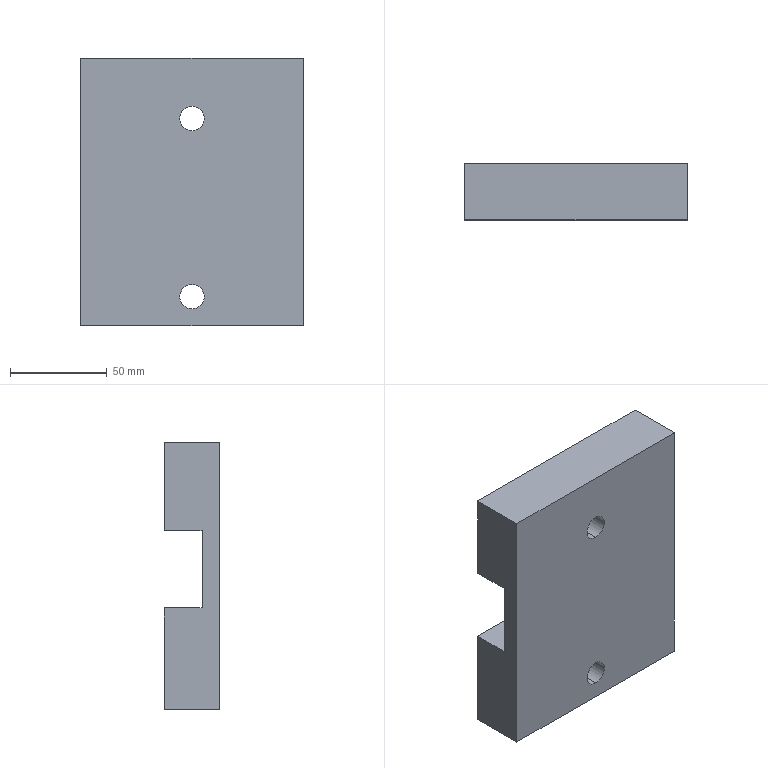Part | SolidWorks | features BaseBody 1 | 1 solid | 20 faces | box 115.385 x 28.846 x 138.462 mm | volume 355349 mm3 | plane 12 | cylinder 8 | commonest cylinder face diameters 12.692 x4 23.077 x4
STEP:
#1=CARTESIAN_POINT('',(207.247,274.423,437.115));
#2=VERTEX_POINT('',#1);
#3=CARTESIAN_POINT('',(207.247,274.423,424.423));
#4=VERTEX_POINT('',#3);
#5=CARTESIAN_POINT('',(207.247,274.423,430.769));
#6=DIRECTION('',(0.,-1.,0.));
#7=DIRECTION('',(0.,0.,-1.));
#8=AXIS2_PLACEMENT_3D('',#5,#6,#7);
#9=CIRCLE('',#8,6.346);
#10=EDGE_CURVE('',#2,#4,#9,.T.);
#11=ORIENTED_EDGE('',*,*,#10,.F.);
#12=CARTESIAN_POINT('',(207.247,258.731,437.115));
#13=VERTEX_POINT('',#12);
#14=CARTESIAN_POINT('',(207.247,287.577,437.115));
#15=DIRECTION('',(0.,-1.,0.));
#16=VECTOR('',#15,1000.);
#17=LINE('',#14,#16);
#18=EDGE_CURVE('',#2,#13,#17,.T.);
#19=ORIENTED_EDGE('',*,*,#18,.T.);
#20=CARTESIAN_POINT('',(207.247,258.731,424.423));
#21=VERTEX_POINT('',#20);
#22=CARTESIAN_POINT('',(207.247,258.731,430.769));
#23=DIRECTION('',(0.,-1.,0.));
#24=DIRECTION('',(0.,0.,-1.));
#25=AXIS2_PLACEMENT_3D('',#22,#23,#24);
#26=CIRCLE('',#25,6.346);
#27=EDGE_CURVE('',#13,#21,#26,.T.);
#28=ORIENTED_EDGE('',*,*,#27,.T.);
#29=CARTESIAN_POINT('',(207.247,287.577,424.423));
#30=DIRECTION('',(0.,-1.,0.));
#31=VECTOR('',#30,1000.);
#32=LINE('',#29,#31);
#33=EDGE_CURVE('',#4,#21,#32,.T.);
#34=ORIENTED_EDGE('',*,*,#33,.F.);
#35=EDGE_LOOP('',(#11,#19,#28,#34));
#36=FACE_OUTER_BOUND('',#35,.T.);
#37=CARTESIAN_POINT('',(207.247,287.577,430.769));
#38=DIRECTION('',(0.,-1.,0.));
#39=DIRECTION('',(0.,0.,-1.));
#40=AXIS2_PLACEMENT_3D('',#37,#38,#39);
#41=CYLINDRICAL_SURFACE('',#40,6.346);
#42=ADVANCED_FACE('',(#36),#41,.F.);
#43=CARTESIAN_POINT('',(207.247,274.423,344.808));
#44=VERTEX_POINT('',#43);
#45=CARTESIAN_POINT('',(207.247,274.423,332.115));
#46=VERTEX_POINT('',#45);
#47=CARTESIAN_POINT('',(207.247,274.423,338.462));
#48=DIRECTION('',(0.,-1.,0.));
#49=DIRECTION('',(0.,0.,-1.));
#50=AXIS2_PLACEMENT_3D('',#47,#48,#49);
#51=CIRCLE('',#50,6.346);
#52=EDGE_CURVE('',#44,#46,#51,.T.);
#53=ORIENTED_EDGE('',*,*,#52,.F.);
#54=CARTESIAN_POINT('',(207.247,258.731,344.808));
#55=VERTEX_POINT('',#54);
#56=CARTESIAN_POINT('',(207.247,287.577,344.808));
#57=DIRECTION('',(0.,-1.,0.));
#58=VECTOR('',#57,1000.);
#59=LINE('',#56,#58);
#60=EDGE_CURVE('',#44,#55,#59,.T.);
#61=ORIENTED_EDGE('',*,*,#60,.T.);
#62=CARTESIAN_POINT('',(207.247,258.731,332.115));
#63=VERTEX_POINT('',#62);
#64=CARTESIAN_POINT('',(207.247,258.731,338.462));
#65=DIRECTION('',(0.,-1.,0.));
#66=DIRECTION('',(0.,0.,-1.));
#67=AXIS2_PLACEMENT_3D('',#64,#65,#66);
#68=CIRCLE('',#67,6.346);
#69=EDGE_CURVE('',#55,#63,#68,.T.);
#70=ORIENTED_EDGE('',*,*,#69,.T.);
#71=CARTESIAN_POINT('',(207.247,287.577,332.115));
#72=DIRECTION('',(0.,-1.,0.));
#73=VECTOR('',#72,1000.);
#74=LINE('',#71,#73);
#75=EDGE_CURVE('',#46,#63,#74,.T.);
#76=ORIENTED_EDGE('',*,*,#75,.F.);
#77=EDGE_LOOP('',(#53,#61,#70,#76));
#78=FACE_OUTER_BOUND('',#77,.T.);
#79=CARTESIAN_POINT('',(207.247,287.577,338.462));
#80=DIRECTION('',(0.,-1.,0.));
#81=DIRECTION('',(0.,0.,-1.));
#82=AXIS2_PLACEMENT_3D('',#79,#80,#81);
#83=CYLINDRICAL_SURFACE('',#82,6.346);
#84=ADVANCED_FACE('',(#78),#83,.F.);
#85=CARTESIAN_POINT('',(207.247,287.577,419.231));
#86=VERTEX_POINT('',#85);
#87=CARTESIAN_POINT('',(207.247,287.577,442.308));
#88=VERTEX_POINT('',#87);
#89=CARTESIAN_POINT('',(207.247,287.577,430.769));
#90=DIRECTION('',(0.,1.,0.));
#91=DIRECTION('',(0.,0.,-1.));
#92=AXIS2_PLACEMENT_3D('',#89,#90,#91);
#93=CIRCLE('',#92,11.538);
#94=EDGE_CURVE('',#86,#88,#93,.T.);
#95=ORIENTED_EDGE('',*,*,#94,.T.);
#96=CARTESIAN_POINT('',(207.247,274.423,442.308));
#97=VERTEX_POINT('',#96);
#98=CARTESIAN_POINT('',(207.247,287.577,442.308));
#99=DIRECTION('',(0.,-1.,0.));
#100=VECTOR('',#99,1000.);
#101=LINE('',#98,#100);
#102=EDGE_CURVE('',#88,#97,#101,.T.);
#103=ORIENTED_EDGE('',*,*,#102,.T.);
#104=CARTESIAN_POINT('',(207.247,274.423,419.231));
#105=VERTEX_POINT('',#104);
#106=CARTESIAN_POINT('',(207.247,274.423,430.769));
#107=DIRECTION('',(0.,1.,0.));
#108=DIRECTION('',(0.,0.,-1.));
#109=AXIS2_PLACEMENT_3D('',#106,#107,#108);
#110=CIRCLE('',#109,11.538);
#111=EDGE_CURVE('',#105,#97,#110,.T.);
#112=ORIENTED_EDGE('',*,*,#111,.F.);
#113=CARTESIAN_POINT('',(207.247,287.577,419.231));
#114=DIRECTION('',(0.,-1.,0.));
#115=VECTOR('',#114,1000.);
#116=LINE('',#113,#115);
#117=EDGE_CURVE('',#86,#105,#116,.T.);
#118=ORIENTED_EDGE('',*,*,#117,.F.);
#119=EDGE_LOOP('',(#95,#103,#112,#118));
#120=FACE_OUTER_BOUND('',#119,.T.);
#121=CARTESIAN_POINT('',(207.247,287.577,430.769));
#122=DIRECTION('',(0.,-1.,0.));
#123=DIRECTION('',(0.,0.,-1.));
#124=AXIS2_PLACEMENT_3D('',#121,#122,#123);
#125=CYLINDRICAL_SURFACE('',#124,11.538);
#126=ADVANCED_FACE('',(#120),#125,.F.);
#127=CARTESIAN_POINT('',(207.247,287.577,326.923));
#128=VERTEX_POINT('',#127);
#129=CARTESIAN_POINT('',(207.247,287.577,350.));
#130=VERTEX_POINT('',#129);
#131=CARTESIAN_POINT('',(207.247,287.577,338.462));
#132=DIRECTION('',(0.,1.,0.));
#133=DIRECTION('',(0.,0.,-1.));
#134=AXIS2_PLACEMENT_3D('',#131,#132,#133);
#135=CIRCLE('',#134,11.538);
#136=EDGE_CURVE('',#128,#130,#135,.T.);
#137=ORIENTED_EDGE('',*,*,#136,.T.);
#138=CARTESIAN_POINT('',(207.247,274.423,350.));
#139=VERTEX_POINT('',#138);
#140=CARTESIAN_POINT('',(207.247,287.577,350.));
#141=DIRECTION('',(0.,-1.,0.));
#142=VECTOR('',#141,1000.);
#143=LINE('',#140,#142);
#144=EDGE_CURVE('',#130,#139,#143,.T.);
#145=ORIENTED_EDGE('',*,*,#144,.T.);
#146=CARTESIAN_POINT('',(207.247,274.423,326.923));
#147=VERTEX_POINT('',#146);
#148=CARTESIAN_POINT('',(207.247,274.423,338.462));
#149=DIRECTION('',(0.,1.,0.));
#150=DIRECTION('',(0.,0.,-1.));
#151=AXIS2_PLACEMENT_3D('',#148,#149,#150);
#152=CIRCLE('',#151,11.538);
#153=EDGE_CURVE('',#147,#139,#152,.T.);
#154=ORIENTED_EDGE('',*,*,#153,.F.);
#155=CARTESIAN_POINT('',(207.247,287.577,326.923));
#156=DIRECTION('',(0.,-1.,0.));
#157=VECTOR('',#156,1000.);
#158=LINE('',#155,#157);
#159=EDGE_CURVE('',#128,#147,#158,.T.);
#160=ORIENTED_EDGE('',*,*,#159,.F.);
#161=EDGE_LOOP('',(#137,#145,#154,#160));
#162=FACE_OUTER_BOUND('',#161,.T.);
#163=CARTESIAN_POINT('',(207.247,287.577,338.462));
#164=DIRECTION('',(0.,-1.,0.));
#165=DIRECTION('',(0.,0.,-1.));
#166=AXIS2_PLACEMENT_3D('',#163,#164,#165);
#167=CYLINDRICAL_SURFACE('',#166,11.538);
#168=ADVANCED_FACE('',(#162),#167,.F.);
#169=CARTESIAN_POINT('',(207.247,258.731,430.769));
#170=DIRECTION('',(0.,-1.,0.));
#171=DIRECTION('',(0.,0.,-1.));
#172=AXIS2_PLACEMENT_3D('',#169,#170,#171);
#173=CIRCLE('',#172,6.346);
#174=EDGE_CURVE('',#21,#13,#173,.T.);
#175=ORIENTED_EDGE('',*,*,#174,.F.);
#176=ORIENTED_EDGE('',*,*,#27,.F.);
#177=EDGE_LOOP('',(#175,#176));
#178=FACE_BOUND('',#177,.T.);
#179=CARTESIAN_POINT('',(207.247,258.731,338.462));
#180=DIRECTION('',(0.,-1.,0.));
#181=DIRECTION('',(0.,0.,-1.));
#182=AXIS2_PLACEMENT_3D('',#179,#180,#181);
#183=CIRCLE('',#182,6.346);
#184=EDGE_CURVE('',#63,#55,#183,.T.);
#185=ORIENTED_EDGE('',*,*,#184,.F.);
#186=ORIENTED_EDGE('',*,*,#69,.F.);
#187=EDGE_LOOP('',(#185,#186));
#188=FACE_BOUND('',#187,.T.);
#189=CARTESIAN_POINT('',(149.554,258.731,461.923));
#190=VERTEX_POINT('',#189);
#191=CARTESIAN_POINT('',(264.939,258.731,461.923));
#192=VERTEX_POINT('',#191);
#193=CARTESIAN_POINT('',(264.939,258.731,461.923));
#194=DIRECTION('',(1.,0.,0.));
#195=VECTOR('',#194,1000.);
#196=LINE('',#193,#195);
#197=EDGE_CURVE('',#190,#192,#196,.T.);
#198=ORIENTED_EDGE('',*,*,#197,.F.);
#199=CARTESIAN_POINT('',(149.554,258.731,323.462));
#200=VERTEX_POINT('',#199);
#201=CARTESIAN_POINT('',(149.554,258.731,461.923));
#202=DIRECTION('',(0.,0.,1.));
#203=VECTOR('',#202,1000.);
#204=LINE('',#201,#203);
#205=EDGE_CURVE('',#200,#190,#204,.T.);
#206=ORIENTED_EDGE('',*,*,#205,.F.);
#207=CARTESIAN_POINT('',(264.939,258.731,323.462));
#208=VERTEX_POINT('',#207);
#209=CARTESIAN_POINT('',(264.939,258.731,323.462));
#210=DIRECTION('',(-1.,0.,0.));
#211=VECTOR('',#210,1000.);
#212=LINE('',#209,#211);
#213=EDGE_CURVE('',#208,#200,#212,.T.);
#214=ORIENTED_EDGE('',*,*,#213,.F.);
#215=CARTESIAN_POINT('',(264.939,258.731,461.923));
#216=DIRECTION('',(0.,0.,-1.));
#217=VECTOR('',#216,1000.);
#218=LINE('',#215,#217);
#219=EDGE_CURVE('',#192,#208,#218,.T.);
#220=ORIENTED_EDGE('',*,*,#219,.F.);
#221=EDGE_LOOP('',(#198,#206,#214,#220));
#222=FACE_OUTER_BOUND('',#221,.T.);
#223=CARTESIAN_POINT('',(264.939,258.731,461.923));
#224=DIRECTION('',(0.,1.,0.));
#225=DIRECTION('',(0.,0.,1.));
#226=AXIS2_PLACEMENT_3D('',#223,#224,#225);
#227=PLANE('',#226);
#228=ADVANCED_FACE('',(#178,#188,#222),#227,.F.);
#229=ORIENTED_EDGE('',*,*,#18,.F.);
#230=CARTESIAN_POINT('',(207.247,274.423,430.769));
#231=DIRECTION('',(0.,-1.,0.));
#232=DIRECTION('',(0.,0.,-1.));
#233=AXIS2_PLACEMENT_3D('',#230,#231,#232);
#234=CIRCLE('',#233,6.346);
#235=EDGE_CURVE('',#4,#2,#234,.T.);
#236=ORIENTED_EDGE('',*,*,#235,.F.);
#237=ORIENTED_EDGE('',*,*,#33,.T.);
#238=ORIENTED_EDGE('',*,*,#174,.T.);
#239=EDGE_LOOP('',(#229,#236,#237,#238));
#240=FACE_OUTER_BOUND('',#239,.T.);
#241=CARTESIAN_POINT('',(207.247,287.577,430.769));
#242=DIRECTION('',(0.,-1.,0.));
#243=DIRECTION('',(0.,0.,-1.));
#244=AXIS2_PLACEMENT_3D('',#241,#242,#243);
#245=CYLINDRICAL_SURFACE('',#244,6.346);
#246=ADVANCED_FACE('',(#240),#245,.F.);
#247=ORIENTED_EDGE('',*,*,#60,.F.);
#248=CARTESIAN_POINT('',(207.247,274.423,338.462));
#249=DIRECTION('',(0.,-1.,0.));
#250=DIRECTION('',(0.,0.,-1.));
#251=AXIS2_PLACEMENT_3D('',#248,#249,#250);
#252=CIRCLE('',#251,6.346);
#253=EDGE_CURVE('',#46,#44,#252,.T.);
#254=ORIENTED_EDGE('',*,*,#253,.F.);
#255=ORIENTED_EDGE('',*,*,#75,.T.);
#256=ORIENTED_EDGE('',*,*,#184,.T.);
#257=EDGE_LOOP('',(#247,#254,#255,#256));
#258=FACE_OUTER_BOUND('',#257,.T.);
#259=CARTESIAN_POINT('',(207.247,287.577,338.462));
#260=DIRECTION('',(0.,-1.,0.));
#261=DIRECTION('',(0.,0.,-1.));
#262=AXIS2_PLACEMENT_3D('',#259,#260,#261);
#263=CYLINDRICAL_SURFACE('',#262,6.346);
#264=ADVANCED_FACE('',(#258),#263,.F.);
#265=CARTESIAN_POINT('',(264.939,267.962,416.154));
#266=VERTEX_POINT('',#265);
#267=CARTESIAN_POINT('',(264.939,287.577,416.154));
#268=VERTEX_POINT('',#267);
#269=CARTESIAN_POINT('',(264.939,287.577,416.154));
#270=DIRECTION('',(0.,1.,0.));
#271=VECTOR('',#270,1000.);
#272=LINE('',#269,#271);
#273=EDGE_CURVE('',#266,#268,#272,.T.);
#274=ORIENTED_EDGE('',*,*,#273,.T.);
#275=CARTESIAN_POINT('',(264.939,287.577,461.923));
#276=VERTEX_POINT('',#275);
#277=CARTESIAN_POINT('',(264.939,287.577,323.462));
#278=DIRECTION('',(0.,0.,1.));
#279=VECTOR('',#278,1000.);
#280=LINE('',#277,#279);
#281=EDGE_CURVE('',#268,#276,#280,.T.);
#282=ORIENTED_EDGE('',*,*,#281,.T.);
#283=CARTESIAN_POINT('',(264.939,287.577,461.923));
#284=DIRECTION('',(0.,-1.,0.));
#285=VECTOR('',#284,1000.);
#286=LINE('',#283,#285);
#287=EDGE_CURVE('',#276,#192,#286,.T.);
#288=ORIENTED_EDGE('',*,*,#287,.T.);
#289=ORIENTED_EDGE('',*,*,#219,.T.);
#290=CARTESIAN_POINT('',(264.939,287.577,323.462));
#291=VERTEX_POINT('',#290);
#292=CARTESIAN_POINT('',(264.939,287.577,323.462));
#293=DIRECTION('',(0.,1.,0.));
#294=VECTOR('',#293,1000.);
#295=LINE('',#292,#294);
#296=EDGE_CURVE('',#208,#291,#295,.T.);
#297=ORIENTED_EDGE('',*,*,#296,.T.);
#298=CARTESIAN_POINT('',(264.939,287.577,376.154));
#299=VERTEX_POINT('',#298);
#300=CARTESIAN_POINT('',(264.939,287.577,323.462));
#301=DIRECTION('',(0.,0.,1.));
#302=VECTOR('',#301,1000.);
#303=LINE('',#300,#302);
#304=EDGE_CURVE('',#291,#299,#303,.T.);
#305=ORIENTED_EDGE('',*,*,#304,.T.);
#306=CARTESIAN_POINT('',(264.939,267.962,376.154));
#307=VERTEX_POINT('',#306);
#308=CARTESIAN_POINT('',(264.939,287.577,376.154));
#309=DIRECTION('',(0.,-1.,0.));
#310=VECTOR('',#309,1000.);
#311=LINE('',#308,#310);
#312=EDGE_CURVE('',#299,#307,#311,.T.);
#313=ORIENTED_EDGE('',*,*,#312,.T.);
#314=CARTESIAN_POINT('',(264.939,267.962,323.462));
#315=DIRECTION('',(0.,0.,1.));
#316=VECTOR('',#315,1000.);
#317=LINE('',#314,#316);
#318=EDGE_CURVE('',#307,#266,#317,.T.);
#319=ORIENTED_EDGE('',*,*,#318,.T.);
#320=EDGE_LOOP('',(#274,#282,#288,#289,#297,#305,#313,#319));
#321=FACE_OUTER_BOUND('',#320,.T.);
#322=CARTESIAN_POINT('',(264.939,287.577,323.462));
#323=DIRECTION('',(1.,0.,0.));
#324=DIRECTION('',(0.,0.,-1.));
#325=AXIS2_PLACEMENT_3D('',#322,#323,#324);
#326=PLANE('',#325);
#327=ADVANCED_FACE('',(#321),#326,.T.);
#328=CARTESIAN_POINT('',(149.554,287.577,461.923));
#329=VERTEX_POINT('',#328);
#330=CARTESIAN_POINT('',(264.939,287.577,461.923));
#331=DIRECTION('',(1.,0.,0.));
#332=VECTOR('',#331,1000.);
#333=LINE('',#330,#332);
#334=EDGE_CURVE('',#329,#276,#333,.T.);
#335=ORIENTED_EDGE('',*,*,#334,.F.);
#336=CARTESIAN_POINT('',(149.554,287.577,461.923));
#337=DIRECTION('',(0.,1.,0.));
#338=VECTOR('',#337,1000.);
#339=LINE('',#336,#338);
#340=EDGE_CURVE('',#190,#329,#339,.T.);
#341=ORIENTED_EDGE('',*,*,#340,.F.);
#342=ORIENTED_EDGE('',*,*,#197,.T.);
#343=ORIENTED_EDGE('',*,*,#287,.F.);
#344=EDGE_LOOP('',(#335,#341,#342,#343));
#345=FACE_OUTER_BOUND('',#344,.T.);
#346=CARTESIAN_POINT('',(264.939,287.577,461.923));
#347=DIRECTION('',(0.,0.,-1.));
#348=DIRECTION('',(-1.,0.,0.));
#349=AXIS2_PLACEMENT_3D('',#346,#347,#348);
#350=PLANE('',#349);
#351=ADVANCED_FACE('',(#345),#350,.F.);
#352=CARTESIAN_POINT('',(149.554,267.962,416.154));
#353=VERTEX_POINT('',#352);
#354=CARTESIAN_POINT('',(149.554,287.577,416.154));
#355=VERTEX_POINT('',#354);
#356=CARTESIAN_POINT('',(149.554,287.577,416.154));
#357=DIRECTION('',(0.,1.,0.));
#358=VECTOR('',#357,1000.);
#359=LINE('',#356,#358);
#360=EDGE_CURVE('',#353,#355,#359,.T.);
#361=ORIENTED_EDGE('',*,*,#360,.F.);
#362=CARTESIAN_POINT('',(149.554,267.962,376.154));
#363=VERTEX_POINT('',#362);
#364=CARTESIAN_POINT('',(149.554,267.962,323.462));
#365=DIRECTION('',(0.,0.,1.));
#366=VECTOR('',#365,1000.);
#367=LINE('',#364,#366);
#368=EDGE_CURVE('',#363,#353,#367,.T.);
#369=ORIENTED_EDGE('',*,*,#368,.F.);
#370=CARTESIAN_POINT('',(149.554,287.577,376.154));
#371=VERTEX_POINT('',#370);
#372=CARTESIAN_POINT('',(149.554,287.577,376.154));
#373=DIRECTION('',(0.,-1.,0.));
#374=VECTOR('',#373,1000.);
#375=LINE('',#372,#374);
#376=EDGE_CURVE('',#371,#363,#375,.T.);
#377=ORIENTED_EDGE('',*,*,#376,.F.);
#378=CARTESIAN_POINT('',(149.554,287.577,323.462));
#379=VERTEX_POINT('',#378);
#380=CARTESIAN_POINT('',(149.554,287.577,323.462));
#381=DIRECTION('',(0.,0.,1.));
#382=VECTOR('',#381,1000.);
#383=LINE('',#380,#382);
#384=EDGE_CURVE('',#379,#371,#383,.T.);
#385=ORIENTED_EDGE('',*,*,#384,.F.);
#386=CARTESIAN_POINT('',(149.554,287.577,323.462));
#387=DIRECTION('',(0.,1.,0.));
#388=VECTOR('',#387,1000.);
#389=LINE('',#386,#388);
#390=EDGE_CURVE('',#200,#379,#389,.T.);
#391=ORIENTED_EDGE('',*,*,#390,.F.);
#392=ORIENTED_EDGE('',*,*,#205,.T.);
#393=ORIENTED_EDGE('',*,*,#340,.T.);
#394=CARTESIAN_POINT('',(149.554,287.577,323.462));
#395=DIRECTION('',(0.,0.,1.));
#396=VECTOR('',#395,1000.);
#397=LINE('',#394,#396);
#398=EDGE_CURVE('',#355,#329,#397,.T.);
#399=ORIENTED_EDGE('',*,*,#398,.F.);
#400=EDGE_LOOP('',(#361,#369,#377,#385,#391,#392,#393,#399));
#401=FACE_OUTER_BOUND('',#400,.T.);
#402=CARTESIAN_POINT('',(149.554,287.577,323.462));
#403=DIRECTION('',(1.,0.,0.));
#404=DIRECTION('',(0.,0.,-1.));
#405=AXIS2_PLACEMENT_3D('',#402,#403,#404);
#406=PLANE('',#405);
#407=ADVANCED_FACE('',(#401),#406,.F.);
#408=ORIENTED_EDGE('',*,*,#213,.T.);
#409=ORIENTED_EDGE('',*,*,#390,.T.);
#410=CARTESIAN_POINT('',(264.939,287.577,323.462));
#411=DIRECTION('',(-1.,0.,0.));
#412=VECTOR('',#411,1000.);
#413=LINE('',#410,#412);
#414=EDGE_CURVE('',#291,#379,#413,.T.);
#415=ORIENTED_EDGE('',*,*,#414,.F.);
#416=ORIENTED_EDGE('',*,*,#296,.F.);
#417=EDGE_LOOP('',(#408,#409,#415,#416));
#418=FACE_OUTER_BOUND('',#417,.T.);
#419=CARTESIAN_POINT('',(264.939,258.731,323.462));
#420=DIRECTION('',(0.,0.,1.));
#421=DIRECTION('',(1.,0.,0.));
#422=AXIS2_PLACEMENT_3D('',#419,#420,#421);
#423=PLANE('',#422);
#424=ADVANCED_FACE('',(#418),#423,.F.);
#425=ORIENTED_EDGE('',*,*,#235,.T.);
#426=ORIENTED_EDGE('',*,*,#10,.T.);
#427=EDGE_LOOP('',(#425,#426));
#428=FACE_BOUND('',#427,.T.);
#429=ORIENTED_EDGE('',*,*,#111,.T.);
#430=CARTESIAN_POINT('',(207.247,274.423,430.769));
#431=DIRECTION('',(0.,1.,0.));
#432=DIRECTION('',(0.,0.,-1.));
#433=AXIS2_PLACEMENT_3D('',#430,#431,#432);
#434=CIRCLE('',#433,11.538);
#435=EDGE_CURVE('',#97,#105,#434,.T.);
#436=ORIENTED_EDGE('',*,*,#435,.T.);
#437=EDGE_LOOP('',(#429,#436));
#438=FACE_OUTER_BOUND('',#437,.T.);
#439=CARTESIAN_POINT('',(207.247,274.423,437.115));
#440=DIRECTION('',(0.,1.,0.));
#441=DIRECTION('',(0.,0.,1.));
#442=AXIS2_PLACEMENT_3D('',#439,#440,#441);
#443=PLANE('',#442);
#444=ADVANCED_FACE('',(#428,#438),#443,.T.);
#445=ORIENTED_EDGE('',*,*,#253,.T.);
#446=ORIENTED_EDGE('',*,*,#52,.T.);
#447=EDGE_LOOP('',(#445,#446));
#448=FACE_BOUND('',#447,.T.);
#449=ORIENTED_EDGE('',*,*,#153,.T.);
#450=CARTESIAN_POINT('',(207.247,274.423,338.462));
#451=DIRECTION('',(0.,1.,0.));
#452=DIRECTION('',(0.,0.,-1.));
#453=AXIS2_PLACEMENT_3D('',#450,#451,#452);
#454=CIRCLE('',#453,11.538);
#455=EDGE_CURVE('',#139,#147,#454,.T.);
#456=ORIENTED_EDGE('',*,*,#455,.T.);
#457=EDGE_LOOP('',(#449,#456));
#458=FACE_OUTER_BOUND('',#457,.T.);
#459=CARTESIAN_POINT('',(207.247,274.423,344.808));
#460=DIRECTION('',(0.,1.,0.));
#461=DIRECTION('',(0.,0.,1.));
#462=AXIS2_PLACEMENT_3D('',#459,#460,#461);
#463=PLANE('',#462);
#464=ADVANCED_FACE('',(#448,#458),#463,.T.);
#465=ORIENTED_EDGE('',*,*,#94,.F.);
#466=CARTESIAN_POINT('',(207.247,287.577,430.769));
#467=DIRECTION('',(0.,1.,0.));
#468=DIRECTION('',(0.,0.,-1.));
#469=AXIS2_PLACEMENT_3D('',#466,#467,#468);
#470=CIRCLE('',#469,11.538);
#471=EDGE_CURVE('',#88,#86,#470,.T.);
#472=ORIENTED_EDGE('',*,*,#471,.F.);
#473=EDGE_LOOP('',(#465,#472));
#474=FACE_BOUND('',#473,.T.);
#475=CARTESIAN_POINT('',(264.939,287.577,416.154));
#476=DIRECTION('',(1.,0.,0.));
#477=VECTOR('',#476,1000.);
#478=LINE('',#475,#477);
#479=EDGE_CURVE('',#355,#268,#478,.T.);
#480=ORIENTED_EDGE('',*,*,#479,.F.);
#481=ORIENTED_EDGE('',*,*,#398,.T.);
#482=ORIENTED_EDGE('',*,*,#334,.T.);
#483=ORIENTED_EDGE('',*,*,#281,.F.);
#484=EDGE_LOOP('',(#480,#481,#482,#483));
#485=FACE_OUTER_BOUND('',#484,.T.);
#486=CARTESIAN_POINT('',(264.939,287.577,418.077));
#487=DIRECTION('',(0.,-1.,0.));
#488=DIRECTION('',(0.,0.,-1.));
#489=AXIS2_PLACEMENT_3D('',#486,#487,#488);
#490=PLANE('',#489);
#491=ADVANCED_FACE('',(#474,#485),#490,.F.);
#492=CARTESIAN_POINT('',(264.939,267.962,416.154));
#493=DIRECTION('',(1.,0.,0.));
#494=VECTOR('',#493,1000.);
#495=LINE('',#492,#494);
#496=EDGE_CURVE('',#353,#266,#495,.T.);
#497=ORIENTED_EDGE('',*,*,#496,.F.);
#498=ORIENTED_EDGE('',*,*,#360,.T.);
#499=ORIENTED_EDGE('',*,*,#479,.T.);
#500=ORIENTED_EDGE('',*,*,#273,.F.);
#501=EDGE_LOOP('',(#497,#498,#499,#500));
#502=FACE_OUTER_BOUND('',#501,.T.);
#503=CARTESIAN_POINT('',(264.939,267.962,416.154));
#504=DIRECTION('',(0.,0.,1.));
#505=DIRECTION('',(1.,0.,0.));
#506=AXIS2_PLACEMENT_3D('',#503,#504,#505);
#507=PLANE('',#506);
#508=ADVANCED_FACE('',(#502),#507,.F.);
#509=CARTESIAN_POINT('',(264.939,267.962,376.154));
#510=DIRECTION('',(1.,0.,0.));
#511=VECTOR('',#510,1000.);
#512=LINE('',#509,#511);
#513=EDGE_CURVE('',#363,#307,#512,.T.);
#514=ORIENTED_EDGE('',*,*,#513,.F.);
#515=ORIENTED_EDGE('',*,*,#368,.T.);
#516=ORIENTED_EDGE('',*,*,#496,.T.);
#517=ORIENTED_EDGE('',*,*,#318,.F.);
#518=EDGE_LOOP('',(#514,#515,#516,#517));
#519=FACE_OUTER_BOUND('',#518,.T.);
#520=CARTESIAN_POINT('',(264.939,267.962,374.231));
#521=DIRECTION('',(0.,-1.,0.));
#522=DIRECTION('',(0.,0.,-1.));
#523=AXIS2_PLACEMENT_3D('',#520,#521,#522);
#524=PLANE('',#523);
#525=ADVANCED_FACE('',(#519),#524,.F.);
#526=CARTESIAN_POINT('',(264.939,287.577,376.154));
#527=DIRECTION('',(1.,0.,0.));
#528=VECTOR('',#527,1000.);
#529=LINE('',#526,#528);
#530=EDGE_CURVE('',#371,#299,#529,.T.);
#531=ORIENTED_EDGE('',*,*,#530,.F.);
#532=ORIENTED_EDGE('',*,*,#376,.T.);
#533=ORIENTED_EDGE('',*,*,#513,.T.);
#534=ORIENTED_EDGE('',*,*,#312,.F.);
#535=EDGE_LOOP('',(#531,#532,#533,#534));
#536=FACE_OUTER_BOUND('',#535,.T.);
#537=CARTESIAN_POINT('',(264.939,287.577,376.154));
#538=DIRECTION('',(0.,0.,-1.));
#539=DIRECTION('',(-1.,0.,0.));
#540=AXIS2_PLACEMENT_3D('',#537,#538,#539);
#541=PLANE('',#540);
#542=ADVANCED_FACE('',(#536),#541,.F.);
#543=ORIENTED_EDGE('',*,*,#136,.F.);
#544=CARTESIAN_POINT('',(207.247,287.577,338.462));
#545=DIRECTION('',(0.,1.,0.));
#546=DIRECTION('',(0.,0.,-1.));
#547=AXIS2_PLACEMENT_3D('',#544,#545,#546);
#548=CIRCLE('',#547,11.538);
#549=EDGE_CURVE('',#130,#128,#548,.T.);
#550=ORIENTED_EDGE('',*,*,#549,.F.);
#551=EDGE_LOOP('',(#543,#550));
#552=FACE_BOUND('',#551,.T.);
#553=ORIENTED_EDGE('',*,*,#414,.T.);
#554=ORIENTED_EDGE('',*,*,#384,.T.);
#555=ORIENTED_EDGE('',*,*,#530,.T.);
#556=ORIENTED_EDGE('',*,*,#304,.F.);
#557=EDGE_LOOP('',(#553,#554,#555,#556));
#558=FACE_OUTER_BOUND('',#557,.T.);
#559=CARTESIAN_POINT('',(264.939,287.577,323.462));
#560=DIRECTION('',(0.,-1.,0.));
#561=DIRECTION('',(0.,0.,-1.));
#562=AXIS2_PLACEMENT_3D('',#559,#560,#561);
#563=PLANE('',#562);
#564=ADVANCED_FACE('',(#552,#558),#563,.F.);
#565=ORIENTED_EDGE('',*,*,#102,.F.);
#566=ORIENTED_EDGE('',*,*,#471,.T.);
#567=ORIENTED_EDGE('',*,*,#117,.T.);
#568=ORIENTED_EDGE('',*,*,#435,.F.);
#569=EDGE_LOOP('',(#565,#566,#567,#568));
#570=FACE_OUTER_BOUND('',#569,.T.);
#571=CARTESIAN_POINT('',(207.247,287.577,430.769));
#572=DIRECTION('',(0.,-1.,0.));
#573=DIRECTION('',(0.,0.,-1.));
#574=AXIS2_PLACEMENT_3D('',#571,#572,#573);
#575=CYLINDRICAL_SURFACE('',#574,11.538);
#576=ADVANCED_FACE('',(#570),#575,.F.);
#577=ORIENTED_EDGE('',*,*,#144,.F.);
#578=ORIENTED_EDGE('',*,*,#549,.T.);
#579=ORIENTED_EDGE('',*,*,#159,.T.);
#580=ORIENTED_EDGE('',*,*,#455,.F.);
#581=EDGE_LOOP('',(#577,#578,#579,#580));
#582=FACE_OUTER_BOUND('',#581,.T.);
#583=CARTESIAN_POINT('',(207.247,287.577,338.462));
#584=DIRECTION('',(0.,-1.,0.));
#585=DIRECTION('',(0.,0.,-1.));
#586=AXIS2_PLACEMENT_3D('',#583,#584,#585);
#587=CYLINDRICAL_SURFACE('',#586,11.538);
#588=ADVANCED_FACE('',(#582),#587,.F.);
#589=CLOSED_SHELL('',(#42,#84,#126,#168,#228,#246,#264,#327,#351,#407,#424,#444,#464,#491,#508,#525,#542,#564,#576,#588));
#590=MANIFOLD_SOLID_BREP('',#589);
#591=CARTESIAN_POINT('',(0.,0.,0.));
#592=DIRECTION('',(0.,0.,1.));
#593=DIRECTION('',(1.,0.,0.));
#594=AXIS2_PLACEMENT_3D('',#591,#592,#593);
#595=(LENGTH_UNIT()NAMED_UNIT(*)SI_UNIT(.MILLI.,.METRE.));
#596=UNCERTAINTY_MEASURE_WITH_UNIT(LENGTH_MEASURE(0.00001),#595,'','');
#597=(NAMED_UNIT(*)PLANE_ANGLE_UNIT()SI_UNIT($,.RADIAN.));
#598=(NAMED_UNIT(*)SI_UNIT($,.STERADIAN.)SOLID_ANGLE_UNIT());
#599=(GEOMETRIC_REPRESENTATION_CONTEXT(3)GLOBAL_UNCERTAINTY_ASSIGNED_CONTEXT((#596))GLOBAL_UNIT_ASSIGNED_CONTEXT((#595,#597,#598))REPRESENTATION_CONTEXT('',''));
#600=ADVANCED_BREP_SHAPE_REPRESENTATION('',(#590,#594),#599);